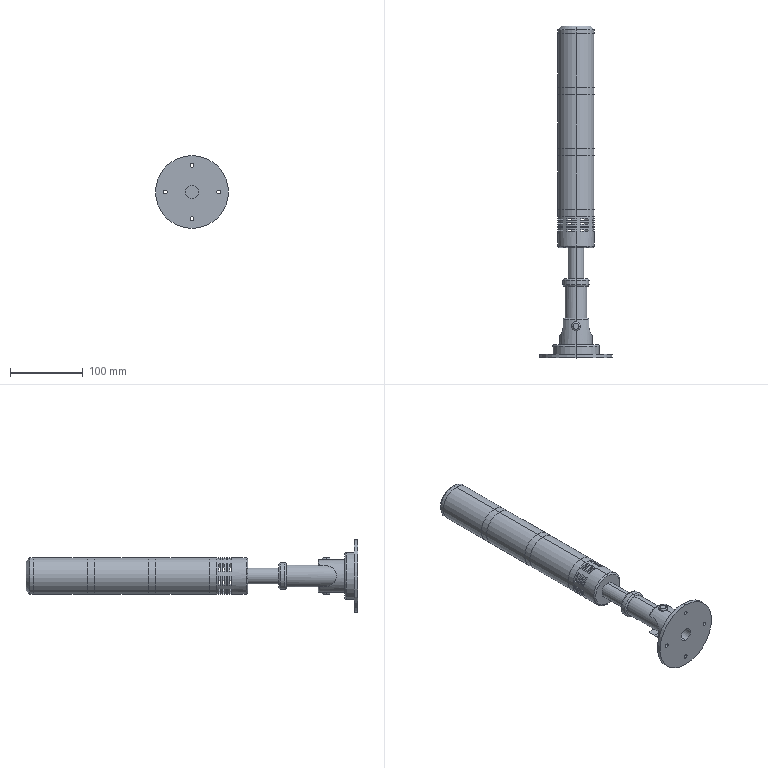Part | SolidWorks | features ICE 17, Fillet 6, BossThin 1, Chamfer 1, CirPattern 1, Extrusion 1, RefAxis 1, RevCut 1 | 8 solids | 221 faces | box 100 x 455.5 x 100 mm | volume 698561 mm3 | plane 158 | cylinder 46 | torus 15 | cone 2 | commonest cylinder face diameters 50 x16 5.2 x8 12 x4 18 x2 21.9 x2 28 x2